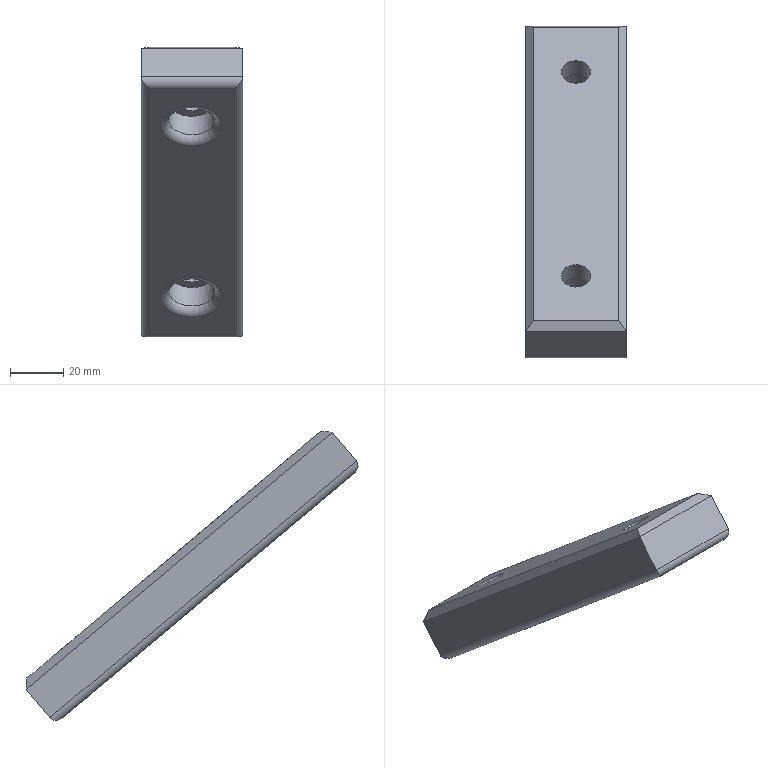Part | NX | features MAIN_BODY 2 | 1 solid | 22 faces | box 38 x 124.608 x 108.584 mm | volume 104106 mm3 | plane 12 | cylinder 8 | torus 2 | commonest cylinder face diameters 6 x4 11 x2 17.5 x2
STEP:
#1=CARTESIAN_POINT('',(-422.,178.621,-110.718));
#2=VERTEX_POINT('',#1);
#3=CARTESIAN_POINT('',(-422.,288.931,-203.28));
#4=VERTEX_POINT('',#3);
#5=CARTESIAN_POINT('',(-422.,291.229,-205.208));
#6=DIRECTION('',(0.,-0.766,0.6428));
#7=VECTOR('',#6,1000.);
#8=LINE('',#5,#7);
#9=EDGE_CURVE('',#2,#4,#8,.F.);
#10=ORIENTED_EDGE('',*,*,#9,.T.);
#11=CARTESIAN_POINT('',(-390.,288.931,-203.28));
#12=VERTEX_POINT('',#11);
#13=CARTESIAN_POINT('',(-387.,288.931,-203.28));
#14=DIRECTION('',(-1.,0.,0.));
#15=VECTOR('',#14,1000.);
#16=LINE('',#13,#15);
#17=EDGE_CURVE('',#4,#12,#16,.F.);
#18=ORIENTED_EDGE('',*,*,#17,.T.);
#19=CARTESIAN_POINT('',(-390.,178.621,-110.718));
#20=VERTEX_POINT('',#19);
#21=CARTESIAN_POINT('',(-390.,176.323,-108.79));
#22=DIRECTION('',(0.,0.766,-0.6428));
#23=VECTOR('',#22,1000.);
#24=LINE('',#21,#23);
#25=EDGE_CURVE('',#12,#20,#24,.F.);
#26=ORIENTED_EDGE('',*,*,#25,.T.);
#27=CARTESIAN_POINT('',(-425.,178.621,-110.718));
#28=DIRECTION('',(1.,0.,0.));
#29=VECTOR('',#28,1000.);
#30=LINE('',#27,#29);
#31=EDGE_CURVE('',#20,#2,#30,.F.);
#32=ORIENTED_EDGE('',*,*,#31,.T.);
#33=EDGE_LOOP('',(#10,#18,#26,#32));
#34=FACE_BOUND('',#33,.T.);
#35=CARTESIAN_POINT('',(-406.,263.077,-181.586));
#36=VERTEX_POINT('',#35);
#37=CARTESIAN_POINT('',(-406.,272.078,-189.139));
#38=DIRECTION('',(0.,0.6428,0.766));
#39=DIRECTION('',(0.,-0.766,0.6428));
#40=AXIS2_PLACEMENT_3D('',#37,#38,#39);
#41=CIRCLE('',#40,11.75);
#42=EDGE_CURVE('',#36,#36,#41,.T.);
#43=ORIENTED_EDGE('',*,*,#42,.T.);
#44=EDGE_LOOP('',(#43));
#45=FACE_BOUND('',#44,.T.);
#46=CARTESIAN_POINT('',(-406.,186.473,-117.307));
#47=VERTEX_POINT('',#46);
#48=CARTESIAN_POINT('',(-406.,195.474,-124.86));
#49=DIRECTION('',(0.,0.6428,0.766));
#50=DIRECTION('',(0.,-0.766,0.6428));
#51=AXIS2_PLACEMENT_3D('',#48,#49,#50);
#52=CIRCLE('',#51,11.75);
#53=EDGE_CURVE('',#47,#47,#52,.T.);
#54=ORIENTED_EDGE('',*,*,#53,.T.);
#55=EDGE_LOOP('',(#54));
#56=FACE_BOUND('',#55,.T.);
#57=CARTESIAN_POINT('',(-425.,176.323,-108.79));
#58=DIRECTION('',(0.,0.6428,0.766));
#59=DIRECTION('',(0.,-0.766,0.6428));
#60=AXIS2_PLACEMENT_3D('',#57,#58,#59);
#61=PLANE('',#60);
#62=ADVANCED_FACE('',(#34,#45,#56),#61,.F.);
#63=CARTESIAN_POINT('',(-400.5,284.934,-173.818));
#64=VERTEX_POINT('',#63);
#65=CARTESIAN_POINT('',(-406.,284.934,-173.818));
#66=DIRECTION('',(0.,-0.6428,-0.766));
#67=DIRECTION('',(1.,0.,0.));
#68=AXIS2_PLACEMENT_3D('',#65,#66,#67);
#69=CIRCLE('',#68,5.5);
#70=EDGE_CURVE('',#64,#64,#69,.T.);
#71=ORIENTED_EDGE('',*,*,#70,.F.);
#72=EDGE_LOOP('',(#71));
#73=FACE_BOUND('',#72,.T.);
#74=CARTESIAN_POINT('',(-406.,284.005,-183.481));
#75=VERTEX_POINT('',#74);
#76=CARTESIAN_POINT('',(-406.,279.792,-179.946));
#77=DIRECTION('',(0.,-0.6428,-0.766));
#78=DIRECTION('',(0.,0.766,-0.6428));
#79=AXIS2_PLACEMENT_3D('',#76,#77,#78);
#80=CIRCLE('',#79,5.5);
#81=EDGE_CURVE('',#75,#75,#80,.T.);
#82=ORIENTED_EDGE('',*,*,#81,.T.);
#83=EDGE_LOOP('',(#82));
#84=FACE_BOUND('',#83,.T.);
#85=CARTESIAN_POINT('',(-406.,272.078,-189.139));
#86=DIRECTION('',(0.,0.6428,0.766));
#87=DIRECTION('',(0.,-0.766,0.6428));
#88=AXIS2_PLACEMENT_3D('',#85,#86,#87);
#89=CYLINDRICAL_SURFACE('',#88,5.5);
#90=ADVANCED_FACE('',(#73,#84),#89,.F.);
#91=CARTESIAN_POINT('',(-390.,191.477,-95.398));
#92=VERTEX_POINT('',#91);
#93=CARTESIAN_POINT('',(-390.,301.787,-187.959));
#94=VERTEX_POINT('',#93);
#95=CARTESIAN_POINT('',(-390.,189.178,-93.469));
#96=DIRECTION('',(0.,0.766,-0.6428));
#97=VECTOR('',#96,1000.);
#98=LINE('',#95,#97);
#99=EDGE_CURVE('',#92,#94,#98,.T.);
#100=ORIENTED_EDGE('',*,*,#99,.T.);
#101=CARTESIAN_POINT('',(-422.,301.787,-187.959));
#102=VERTEX_POINT('',#101);
#103=CARTESIAN_POINT('',(-425.,301.787,-187.959));
#104=DIRECTION('',(-1.,0.,0.));
#105=VECTOR('',#104,1000.);
#106=LINE('',#103,#105);
#107=EDGE_CURVE('',#94,#102,#106,.T.);
#108=ORIENTED_EDGE('',*,*,#107,.T.);
#109=CARTESIAN_POINT('',(-422.,191.477,-95.398));
#110=VERTEX_POINT('',#109);
#111=CARTESIAN_POINT('',(-422.,189.178,-93.469));
#112=DIRECTION('',(0.,-0.766,0.6428));
#113=VECTOR('',#112,1000.);
#114=LINE('',#111,#113);
#115=EDGE_CURVE('',#102,#110,#114,.T.);
#116=ORIENTED_EDGE('',*,*,#115,.T.);
#117=CARTESIAN_POINT('',(-425.,191.477,-95.398));
#118=DIRECTION('',(1.,0.,0.));
#119=VECTOR('',#118,1000.);
#120=LINE('',#117,#119);
#121=EDGE_CURVE('',#110,#92,#120,.T.);
#122=ORIENTED_EDGE('',*,*,#121,.T.);
#123=EDGE_LOOP('',(#100,#108,#116,#122));
#124=FACE_BOUND('',#123,.T.);
#125=CARTESIAN_POINT('',(-400.5,208.33,-109.539));
#126=VERTEX_POINT('',#125);
#127=CARTESIAN_POINT('',(-406.,208.33,-109.539));
#128=DIRECTION('',(0.,0.6428,0.766));
#129=DIRECTION('',(1.,0.,0.));
#130=AXIS2_PLACEMENT_3D('',#127,#128,#129);
#131=CIRCLE('',#130,5.5);
#132=EDGE_CURVE('',#126,#126,#131,.T.);
#133=ORIENTED_EDGE('',*,*,#132,.F.);
#134=EDGE_LOOP('',(#133));
#135=FACE_BOUND('',#134,.T.);
#136=ORIENTED_EDGE('',*,*,#70,.T.);
#137=EDGE_LOOP('',(#136));
#138=FACE_BOUND('',#137,.T.);
#139=CARTESIAN_POINT('',(-425.,189.178,-93.469));
#140=DIRECTION('',(0.,0.6428,0.766));
#141=DIRECTION('',(0.,-0.766,0.6428));
#142=AXIS2_PLACEMENT_3D('',#139,#140,#141);
#143=PLANE('',#142);
#144=ADVANCED_FACE('',(#124,#135,#138),#143,.T.);
#145=CARTESIAN_POINT('',(-425.,178.251,-106.492));
#146=VERTEX_POINT('',#145);
#147=CARTESIAN_POINT('',(-425.,187.25,-95.767));
#148=VERTEX_POINT('',#147);
#149=CARTESIAN_POINT('',(-425.,176.323,-108.79));
#150=DIRECTION('',(0.,0.6428,0.766));
#151=VECTOR('',#150,1000.);
#152=LINE('',#149,#151);
#153=EDGE_CURVE('',#146,#148,#152,.T.);
#154=ORIENTED_EDGE('',*,*,#153,.T.);
#155=CARTESIAN_POINT('',(-425.,302.157,-192.186));
#156=VERTEX_POINT('',#155);
#157=CARTESIAN_POINT('',(-425.,302.157,-192.186));
#158=DIRECTION('',(0.,0.766,-0.6428));
#159=VECTOR('',#158,1000.);
#160=LINE('',#157,#159);
#161=EDGE_CURVE('',#148,#156,#160,.T.);
#162=ORIENTED_EDGE('',*,*,#161,.T.);
#163=CARTESIAN_POINT('',(-425.,293.158,-202.91));
#164=VERTEX_POINT('',#163);
#165=CARTESIAN_POINT('',(-425.,291.229,-205.208));
#166=DIRECTION('',(0.,0.6428,0.766));
#167=VECTOR('',#166,1000.);
#168=LINE('',#165,#167);
#169=EDGE_CURVE('',#164,#156,#168,.T.);
#170=ORIENTED_EDGE('',*,*,#169,.F.);
#171=CARTESIAN_POINT('',(-425.,178.251,-106.492));
#172=DIRECTION('',(0.,-0.766,0.6428));
#173=VECTOR('',#172,1000.);
#174=LINE('',#171,#173);
#175=EDGE_CURVE('',#164,#146,#174,.T.);
#176=ORIENTED_EDGE('',*,*,#175,.T.);
#177=EDGE_LOOP('',(#154,#162,#170,#176));
#178=FACE_BOUND('',#177,.T.);
#179=CARTESIAN_POINT('',(-425.,291.229,-205.208));
#180=DIRECTION('',(-1.,0.,0.));
#181=DIRECTION('',(0.,0.766,-0.6428));
#182=AXIS2_PLACEMENT_3D('',#179,#180,#181);
#183=PLANE('',#182);
#184=ADVANCED_FACE('',(#178),#183,.T.);
#185=CARTESIAN_POINT('',(-387.,178.251,-106.492));
#186=VERTEX_POINT('',#185);
#187=CARTESIAN_POINT('',(-387.,187.25,-95.767));
#188=VERTEX_POINT('',#187);
#189=CARTESIAN_POINT('',(-387.,176.323,-108.79));
#190=DIRECTION('',(0.,0.6428,0.766));
#191=VECTOR('',#190,1000.);
#192=LINE('',#189,#191);
#193=EDGE_CURVE('',#186,#188,#192,.T.);
#194=ORIENTED_EDGE('',*,*,#193,.T.);
#195=CARTESIAN_POINT('',(-425.,187.25,-95.767));
#196=DIRECTION('',(-1.,0.,0.));
#197=VECTOR('',#196,1000.);
#198=LINE('',#195,#197);
#199=EDGE_CURVE('',#188,#148,#198,.T.);
#200=ORIENTED_EDGE('',*,*,#199,.T.);
#201=ORIENTED_EDGE('',*,*,#153,.F.);
#202=CARTESIAN_POINT('',(-387.,178.251,-106.492));
#203=DIRECTION('',(1.,0.,0.));
#204=VECTOR('',#203,1000.);
#205=LINE('',#202,#204);
#206=EDGE_CURVE('',#146,#186,#205,.T.);
#207=ORIENTED_EDGE('',*,*,#206,.T.);
#208=EDGE_LOOP('',(#194,#200,#201,#207));
#209=FACE_BOUND('',#208,.T.);
#210=CARTESIAN_POINT('',(-425.,176.323,-108.79));
#211=DIRECTION('',(0.,-0.766,0.6428));
#212=DIRECTION('',(-1.,0.,0.));
#213=AXIS2_PLACEMENT_3D('',#210,#211,#212);
#214=PLANE('',#213);
#215=ADVANCED_FACE('',(#209),#214,.T.);
#216=CARTESIAN_POINT('',(-387.,293.158,-202.91));
#217=VERTEX_POINT('',#216);
#218=CARTESIAN_POINT('',(-387.,302.157,-192.186));
#219=VERTEX_POINT('',#218);
#220=CARTESIAN_POINT('',(-387.,291.229,-205.208));
#221=DIRECTION('',(0.,0.6428,0.766));
#222=VECTOR('',#221,1000.);
#223=LINE('',#220,#222);
#224=EDGE_CURVE('',#217,#219,#223,.T.);
#225=ORIENTED_EDGE('',*,*,#224,.T.);
#226=CARTESIAN_POINT('',(-387.,187.25,-95.767));
#227=DIRECTION('',(0.,-0.766,0.6428));
#228=VECTOR('',#227,1000.);
#229=LINE('',#226,#228);
#230=EDGE_CURVE('',#219,#188,#229,.T.);
#231=ORIENTED_EDGE('',*,*,#230,.T.);
#232=ORIENTED_EDGE('',*,*,#193,.F.);
#233=CARTESIAN_POINT('',(-387.,293.158,-202.91));
#234=DIRECTION('',(0.,0.766,-0.6428));
#235=VECTOR('',#234,1000.);
#236=LINE('',#233,#235);
#237=EDGE_CURVE('',#186,#217,#236,.T.);
#238=ORIENTED_EDGE('',*,*,#237,.T.);
#239=EDGE_LOOP('',(#225,#231,#232,#238));
#240=FACE_BOUND('',#239,.T.);
#241=CARTESIAN_POINT('',(-387.,176.323,-108.79));
#242=DIRECTION('',(1.,0.,0.));
#243=DIRECTION('',(0.,-0.766,0.6428));
#244=AXIS2_PLACEMENT_3D('',#241,#242,#243);
#245=PLANE('',#244);
#246=ADVANCED_FACE('',(#240),#245,.T.);
#247=ORIENTED_EDGE('',*,*,#169,.T.);
#248=CARTESIAN_POINT('',(-387.,302.157,-192.186));
#249=DIRECTION('',(1.,0.,0.));
#250=VECTOR('',#249,1000.);
#251=LINE('',#248,#250);
#252=EDGE_CURVE('',#156,#219,#251,.T.);
#253=ORIENTED_EDGE('',*,*,#252,.T.);
#254=ORIENTED_EDGE('',*,*,#224,.F.);
#255=CARTESIAN_POINT('',(-425.,293.158,-202.91));
#256=DIRECTION('',(-1.,0.,0.));
#257=VECTOR('',#256,1000.);
#258=LINE('',#255,#257);
#259=EDGE_CURVE('',#217,#164,#258,.T.);
#260=ORIENTED_EDGE('',*,*,#259,.T.);
#261=EDGE_LOOP('',(#247,#253,#254,#260));
#262=FACE_BOUND('',#261,.T.);
#263=CARTESIAN_POINT('',(-387.,291.229,-205.208));
#264=DIRECTION('',(0.,0.766,-0.6428));
#265=DIRECTION('',(1.,0.,0.));
#266=AXIS2_PLACEMENT_3D('',#263,#264,#265);
#267=PLANE('',#266);
#268=ADVANCED_FACE('',(#262),#267,.T.);
#269=CARTESIAN_POINT('',(-406.,198.974,-112.132));
#270=VERTEX_POINT('',#269);
#271=CARTESIAN_POINT('',(-406.,203.187,-115.667));
#272=DIRECTION('',(0.,0.6428,0.766));
#273=DIRECTION('',(0.,-0.766,0.6428));
#274=AXIS2_PLACEMENT_3D('',#271,#272,#273);
#275=CIRCLE('',#274,5.5);
#276=EDGE_CURVE('',#270,#270,#275,.F.);
#277=ORIENTED_EDGE('',*,*,#276,.T.);
#278=EDGE_LOOP('',(#277));
#279=FACE_BOUND('',#278,.T.);
#280=ORIENTED_EDGE('',*,*,#132,.T.);
#281=EDGE_LOOP('',(#280));
#282=FACE_BOUND('',#281,.T.);
#283=CARTESIAN_POINT('',(-406.,195.474,-124.86));
#284=DIRECTION('',(0.,0.6428,0.766));
#285=DIRECTION('',(0.,-0.766,0.6428));
#286=AXIS2_PLACEMENT_3D('',#283,#284,#285);
#287=CYLINDRICAL_SURFACE('',#286,5.5);
#288=ADVANCED_FACE('',(#279,#282),#287,.F.);
#289=CARTESIAN_POINT('',(-406.,267.304,-181.216));
#290=VERTEX_POINT('',#289);
#291=CARTESIAN_POINT('',(-406.,274.007,-186.84));
#292=DIRECTION('',(0.,0.6428,0.766));
#293=DIRECTION('',(0.,-0.766,0.6428));
#294=AXIS2_PLACEMENT_3D('',#291,#292,#293);
#295=CIRCLE('',#294,8.75);
#296=EDGE_CURVE('',#290,#290,#295,.F.);
#297=ORIENTED_EDGE('',*,*,#296,.T.);
#298=EDGE_LOOP('',(#297));
#299=FACE_BOUND('',#298,.T.);
#300=CARTESIAN_POINT('',(-397.25,279.792,-179.946));
#301=VERTEX_POINT('',#300);
#302=CARTESIAN_POINT('',(-406.,279.792,-179.946));
#303=DIRECTION('',(0.,-0.6428,-0.766));
#304=DIRECTION('',(1.,0.,0.));
#305=AXIS2_PLACEMENT_3D('',#302,#303,#304);
#306=CIRCLE('',#305,8.75);
#307=EDGE_CURVE('',#301,#301,#306,.T.);
#308=ORIENTED_EDGE('',*,*,#307,.F.);
#309=EDGE_LOOP('',(#308));
#310=FACE_BOUND('',#309,.T.);
#311=CARTESIAN_POINT('',(-406.,265.65,-196.799));
#312=DIRECTION('',(0.,0.6428,0.766));
#313=DIRECTION('',(0.,-0.766,0.6428));
#314=AXIS2_PLACEMENT_3D('',#311,#312,#313);
#315=CYLINDRICAL_SURFACE('',#314,8.75);
#316=ADVANCED_FACE('',(#299,#310),#315,.F.);
#317=ORIENTED_EDGE('',*,*,#81,.F.);
#318=EDGE_LOOP('',(#317));
#319=FACE_BOUND('',#318,.T.);
#320=ORIENTED_EDGE('',*,*,#307,.T.);
#321=EDGE_LOOP('',(#320));
#322=FACE_BOUND('',#321,.T.);
#323=CARTESIAN_POINT('',(-406.,279.792,-179.946));
#324=DIRECTION('',(0.,-0.6428,-0.766));
#325=DIRECTION('',(0.,0.766,-0.6428));
#326=AXIS2_PLACEMENT_3D('',#323,#324,#325);
#327=PLANE('',#326);
#328=ADVANCED_FACE('',(#319,#322),#327,.T.);
#329=CARTESIAN_POINT('',(-406.,190.699,-116.937));
#330=VERTEX_POINT('',#329);
#331=CARTESIAN_POINT('',(-406.,197.402,-122.562));
#332=DIRECTION('',(0.,0.6428,0.766));
#333=DIRECTION('',(0.,-0.766,0.6428));
#334=AXIS2_PLACEMENT_3D('',#331,#332,#333);
#335=CIRCLE('',#334,8.75);
#336=EDGE_CURVE('',#330,#330,#335,.F.);
#337=ORIENTED_EDGE('',*,*,#336,.T.);
#338=EDGE_LOOP('',(#337));
#339=FACE_BOUND('',#338,.T.);
#340=CARTESIAN_POINT('',(-397.25,203.187,-115.667));
#341=VERTEX_POINT('',#340);
#342=CARTESIAN_POINT('',(-406.,203.187,-115.667));
#343=DIRECTION('',(0.,0.6428,0.766));
#344=DIRECTION('',(1.,0.,0.));
#345=AXIS2_PLACEMENT_3D('',#342,#343,#344);
#346=CIRCLE('',#345,8.75);
#347=EDGE_CURVE('',#341,#341,#346,.T.);
#348=ORIENTED_EDGE('',*,*,#347,.T.);
#349=EDGE_LOOP('',(#348));
#350=FACE_BOUND('',#349,.T.);
#351=CARTESIAN_POINT('',(-406.,189.046,-132.52));
#352=DIRECTION('',(0.,0.6428,0.766));
#353=DIRECTION('',(0.,-0.766,0.6428));
#354=AXIS2_PLACEMENT_3D('',#351,#352,#353);
#355=CYLINDRICAL_SURFACE('',#354,8.75);
#356=ADVANCED_FACE('',(#339,#350),#355,.F.);
#357=ORIENTED_EDGE('',*,*,#347,.F.);
#358=EDGE_LOOP('',(#357));
#359=FACE_BOUND('',#358,.T.);
#360=ORIENTED_EDGE('',*,*,#276,.F.);
#361=EDGE_LOOP('',(#360));
#362=FACE_BOUND('',#361,.T.);
#363=CARTESIAN_POINT('',(-406.,203.187,-115.667));
#364=DIRECTION('',(0.,0.6428,0.766));
#365=DIRECTION('',(0.,-0.766,0.6428));
#366=AXIS2_PLACEMENT_3D('',#363,#364,#365);
#367=PLANE('',#366);
#368=ADVANCED_FACE('',(#359,#362),#367,.F.);
#369=CARTESIAN_POINT('',(-422.,180.549,-108.42));
#370=DIRECTION('',(-0.7071,0.5417,-0.4545));
#371=DIRECTION('',(-0.7071,-0.5417,0.4545));
#372=AXIS2_PLACEMENT_3D('',#369,#370,#371);
#373=ELLIPSE('',#372,4.243,3.);
#374=EDGE_CURVE('',#2,#146,#373,.T.);
#375=ORIENTED_EDGE('',*,*,#374,.F.);
#376=ORIENTED_EDGE('',*,*,#31,.F.);
#377=CARTESIAN_POINT('',(-390.,180.549,-108.42));
#378=DIRECTION('',(-0.7071,-0.5417,0.4545));
#379=DIRECTION('',(-0.7071,0.5417,-0.4545));
#380=AXIS2_PLACEMENT_3D('',#377,#378,#379);
#381=ELLIPSE('',#380,4.243,3.);
#382=EDGE_CURVE('',#186,#20,#381,.F.);
#383=ORIENTED_EDGE('',*,*,#382,.F.);
#384=ORIENTED_EDGE('',*,*,#206,.F.);
#385=EDGE_LOOP('',(#375,#376,#383,#384));
#386=FACE_BOUND('',#385,.T.);
#387=CARTESIAN_POINT('',(-425.,180.549,-108.42));
#388=DIRECTION('',(-1.,0.,0.));
#389=DIRECTION('',(0.,0.766,-0.6428));
#390=AXIS2_PLACEMENT_3D('',#387,#388,#389);
#391=CYLINDRICAL_SURFACE('',#390,3.);
#392=ADVANCED_FACE('',(#386),#391,.T.);
#393=ORIENTED_EDGE('',*,*,#382,.T.);
#394=ORIENTED_EDGE('',*,*,#25,.F.);
#395=CARTESIAN_POINT('',(-390.,290.86,-200.982));
#396=DIRECTION('',(0.7071,-0.5417,0.4545));
#397=DIRECTION('',(-0.7071,-0.5417,0.4545));
#398=AXIS2_PLACEMENT_3D('',#395,#396,#397);
#399=ELLIPSE('',#398,4.243,3.);
#400=EDGE_CURVE('',#217,#12,#399,.F.);
#401=ORIENTED_EDGE('',*,*,#400,.F.);
#402=ORIENTED_EDGE('',*,*,#237,.F.);
#403=EDGE_LOOP('',(#393,#394,#401,#402));
#404=FACE_BOUND('',#403,.T.);
#405=CARTESIAN_POINT('',(-390.,178.251,-106.492));
#406=DIRECTION('',(0.,-0.766,0.6428));
#407=DIRECTION('',(-1.,0.,0.));
#408=AXIS2_PLACEMENT_3D('',#405,#406,#407);
#409=CYLINDRICAL_SURFACE('',#408,3.);
#410=ADVANCED_FACE('',(#404),#409,.T.);
#411=ORIENTED_EDGE('',*,*,#374,.T.);
#412=ORIENTED_EDGE('',*,*,#175,.F.);
#413=CARTESIAN_POINT('',(-422.,290.86,-200.982));
#414=DIRECTION('',(0.7071,0.5417,-0.4545));
#415=DIRECTION('',(-0.7071,0.5417,-0.4545));
#416=AXIS2_PLACEMENT_3D('',#413,#414,#415);
#417=ELLIPSE('',#416,4.243,3.);
#418=EDGE_CURVE('',#4,#164,#417,.T.);
#419=ORIENTED_EDGE('',*,*,#418,.F.);
#420=ORIENTED_EDGE('',*,*,#9,.F.);
#421=EDGE_LOOP('',(#411,#412,#419,#420));
#422=FACE_BOUND('',#421,.T.);
#423=CARTESIAN_POINT('',(-422.,293.158,-202.91));
#424=DIRECTION('',(0.,0.766,-0.6428));
#425=DIRECTION('',(1.,0.,0.));
#426=AXIS2_PLACEMENT_3D('',#423,#424,#425);
#427=CYLINDRICAL_SURFACE('',#426,3.);
#428=ADVANCED_FACE('',(#422),#427,.T.);
#429=ORIENTED_EDGE('',*,*,#400,.T.);
#430=ORIENTED_EDGE('',*,*,#17,.F.);
#431=ORIENTED_EDGE('',*,*,#418,.T.);
#432=ORIENTED_EDGE('',*,*,#259,.F.);
#433=EDGE_LOOP('',(#429,#430,#431,#432));
#434=FACE_BOUND('',#433,.T.);
#435=CARTESIAN_POINT('',(-387.,290.86,-200.982));
#436=DIRECTION('',(1.,0.,0.));
#437=DIRECTION('',(0.,-0.766,0.6428));
#438=AXIS2_PLACEMENT_3D('',#435,#436,#437);
#439=CYLINDRICAL_SURFACE('',#438,3.);
#440=ADVANCED_FACE('',(#434),#439,.T.);
#441=ORIENTED_EDGE('',*,*,#42,.F.);
#442=EDGE_LOOP('',(#441));
#443=FACE_BOUND('',#442,.T.);
#444=ORIENTED_EDGE('',*,*,#296,.F.);
#445=EDGE_LOOP('',(#444));
#446=FACE_BOUND('',#445,.T.);
#447=CARTESIAN_POINT('',(-406.,274.007,-186.84));
#448=DIRECTION('',(0.,0.6428,0.766));
#449=DIRECTION('',(0.,-0.766,0.6428));
#450=AXIS2_PLACEMENT_3D('',#447,#448,#449);
#451=TOROIDAL_SURFACE('',#450,11.75,3.);
#452=ADVANCED_FACE('',(#443,#446),#451,.T.);
#453=ORIENTED_EDGE('',*,*,#336,.F.);
#454=EDGE_LOOP('',(#453));
#455=FACE_BOUND('',#454,.T.);
#456=ORIENTED_EDGE('',*,*,#53,.F.);
#457=EDGE_LOOP('',(#456));
#458=FACE_BOUND('',#457,.T.);
#459=CARTESIAN_POINT('',(-406.,197.402,-122.562));
#460=DIRECTION('',(0.,0.6428,0.766));
#461=DIRECTION('',(0.,-0.766,0.6428));
#462=AXIS2_PLACEMENT_3D('',#459,#460,#461);
#463=TOROIDAL_SURFACE('',#462,11.75,3.);
#464=ADVANCED_FACE('',(#455,#458),#463,.T.);
#465=CARTESIAN_POINT('',(-423.,190.068,-95.521));
#466=DIRECTION('',(-0.5774,-0.8134,-0.07116));
#467=VECTOR('',#466,1000.);
#468=LINE('',#465,#467);
#469=EDGE_CURVE('',#148,#110,#468,.F.);
#470=ORIENTED_EDGE('',*,*,#469,.F.);
#471=ORIENTED_EDGE('',*,*,#199,.F.);
#472=CARTESIAN_POINT('',(-389.,190.068,-95.521));
#473=DIRECTION('',(0.5774,-0.8134,-0.07116));
#474=VECTOR('',#473,1000.);
#475=LINE('',#472,#474);
#476=EDGE_CURVE('',#92,#188,#475,.T.);
#477=ORIENTED_EDGE('',*,*,#476,.F.);
#478=ORIENTED_EDGE('',*,*,#121,.F.);
#479=EDGE_LOOP('',(#470,#471,#477,#478));
#480=FACE_BOUND('',#479,.T.);
#481=CARTESIAN_POINT('',(-425.,191.477,-95.398));
#482=DIRECTION('',(0.,0.08716,-0.9962));
#483=DIRECTION('',(0.,0.9962,0.08716));
#484=AXIS2_PLACEMENT_3D('',#481,#482,#483);
#485=PLANE('',#484);
#486=ADVANCED_FACE('',(#480),#485,.F.);
#487=ORIENTED_EDGE('',*,*,#476,.T.);
#488=ORIENTED_EDGE('',*,*,#230,.F.);
#489=CARTESIAN_POINT('',(-439.,295.747,-118.926));
#490=DIRECTION('',(-0.5774,-0.07116,0.8134));
#491=VECTOR('',#490,1000.);
#492=LINE('',#489,#491);
#493=EDGE_CURVE('',#94,#219,#492,.F.);
#494=ORIENTED_EDGE('',*,*,#493,.F.);
#495=ORIENTED_EDGE('',*,*,#99,.F.);
#496=EDGE_LOOP('',(#487,#488,#494,#495));
#497=FACE_BOUND('',#496,.T.);
#498=CARTESIAN_POINT('',(-390.,189.178,-93.469));
#499=DIRECTION('',(-0.7071,-0.4545,-0.5417));
#500=DIRECTION('',(0.7071,-0.4545,-0.5417));
#501=AXIS2_PLACEMENT_3D('',#498,#499,#500);
#502=PLANE('',#501);
#503=ADVANCED_FACE('',(#497),#502,.F.);
#504=ORIENTED_EDGE('',*,*,#469,.T.);
#505=ORIENTED_EDGE('',*,*,#115,.F.);
#506=CARTESIAN_POINT('',(-373.,295.747,-118.926));
#507=DIRECTION('',(-0.5774,0.07116,-0.8134));
#508=VECTOR('',#507,1000.);
#509=LINE('',#506,#508);
#510=EDGE_CURVE('',#156,#102,#509,.F.);
#511=ORIENTED_EDGE('',*,*,#510,.F.);
#512=ORIENTED_EDGE('',*,*,#161,.F.);
#513=EDGE_LOOP('',(#504,#505,#511,#512));
#514=FACE_BOUND('',#513,.T.);
#515=CARTESIAN_POINT('',(-422.,189.178,-93.469));
#516=DIRECTION('',(0.7071,-0.4545,-0.5417));
#517=DIRECTION('',(0.7071,0.4545,0.5417));
#518=AXIS2_PLACEMENT_3D('',#515,#516,#517);
#519=PLANE('',#518);
#520=ADVANCED_FACE('',(#514),#519,.F.);
#521=ORIENTED_EDGE('',*,*,#493,.T.);
#522=ORIENTED_EDGE('',*,*,#252,.F.);
#523=ORIENTED_EDGE('',*,*,#510,.T.);
#524=ORIENTED_EDGE('',*,*,#107,.F.);
#525=EDGE_LOOP('',(#521,#522,#523,#524));
#526=FACE_BOUND('',#525,.T.);
#527=CARTESIAN_POINT('',(-425.,301.787,-187.959));
#528=DIRECTION('',(0.,-0.9962,-0.08716));
#529=DIRECTION('',(0.,0.08716,-0.9962));
#530=AXIS2_PLACEMENT_3D('',#527,#528,#529);
#531=PLANE('',#530);
#532=ADVANCED_FACE('',(#526),#531,.F.);
#533=CLOSED_SHELL('',(#62,#90,#144,#184,#215,#246,#268,#288,#316,#328,#356,#368,#392,#410,#428,#440,#452,#464,#486,#503,#520,#532));
#534=MANIFOLD_SOLID_BREP('',#533);
#535=(LENGTH_UNIT()NAMED_UNIT(*)SI_UNIT(.MILLI.,.METRE.));
#536=UNCERTAINTY_MEASURE_WITH_UNIT(LENGTH_MEASURE(0.00001),#535,'','');
#537=(NAMED_UNIT(*)PLANE_ANGLE_UNIT()SI_UNIT($,.RADIAN.));
#538=(NAMED_UNIT(*)SI_UNIT($,.STERADIAN.)SOLID_ANGLE_UNIT());
#539=(GEOMETRIC_REPRESENTATION_CONTEXT(3)GLOBAL_UNCERTAINTY_ASSIGNED_CONTEXT((#536))GLOBAL_UNIT_ASSIGNED_CONTEXT((#535,#537,#538))REPRESENTATION_CONTEXT('',''));
#540=ADVANCED_BREP_SHAPE_REPRESENTATION('',(#534),#539);